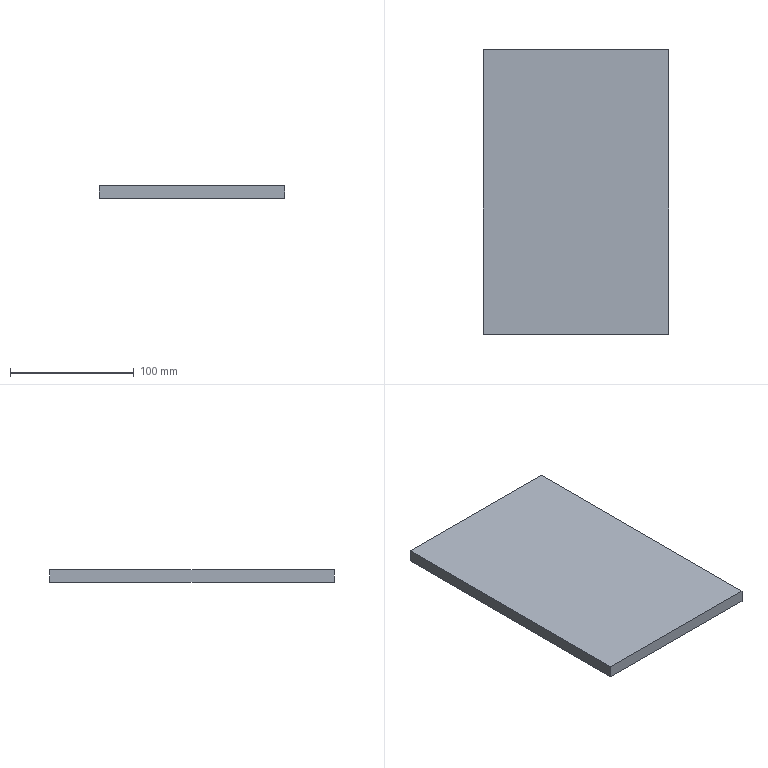Part | SolidWorks | features Extrusion 1 | 1 solid | 6 faces | box 150 x 230 x 10 mm | volume 345000 mm3 | plane 6
STEP:
#1=CARTESIAN_POINT('',(-75.,115.,-5.));
#2=VERTEX_POINT('',#1);
#3=CARTESIAN_POINT('',(-75.,-115.,-5.));
#4=VERTEX_POINT('',#3);
#5=CARTESIAN_POINT('',(-75.,-115.,-5.));
#6=DIRECTION('',(0.,-1.,0.));
#7=VECTOR('',#6,1000.);
#8=LINE('',#5,#7);
#9=EDGE_CURVE('',#2,#4,#8,.T.);
#10=ORIENTED_EDGE('',*,*,#9,.T.);
#11=CARTESIAN_POINT('',(-75.,-115.,5.));
#12=VERTEX_POINT('',#11);
#13=CARTESIAN_POINT('',(-75.,-115.,5.));
#14=DIRECTION('',(0.,0.,-1.));
#15=VECTOR('',#14,1000.);
#16=LINE('',#13,#15);
#17=EDGE_CURVE('',#12,#4,#16,.T.);
#18=ORIENTED_EDGE('',*,*,#17,.F.);
#19=CARTESIAN_POINT('',(-75.,115.,5.));
#20=VERTEX_POINT('',#19);
#21=CARTESIAN_POINT('',(-75.,-115.,5.));
#22=DIRECTION('',(0.,-1.,0.));
#23=VECTOR('',#22,1000.);
#24=LINE('',#21,#23);
#25=EDGE_CURVE('',#20,#12,#24,.T.);
#26=ORIENTED_EDGE('',*,*,#25,.F.);
#27=CARTESIAN_POINT('',(-75.,115.,5.));
#28=DIRECTION('',(0.,0.,-1.));
#29=VECTOR('',#28,1000.);
#30=LINE('',#27,#29);
#31=EDGE_CURVE('',#20,#2,#30,.T.);
#32=ORIENTED_EDGE('',*,*,#31,.T.);
#33=EDGE_LOOP('',(#10,#18,#26,#32));
#34=FACE_OUTER_BOUND('',#33,.T.);
#35=CARTESIAN_POINT('',(-75.,-115.,5.));
#36=DIRECTION('',(1.,0.,0.));
#37=DIRECTION('',(0.,0.,-1.));
#38=AXIS2_PLACEMENT_3D('',#35,#36,#37);
#39=PLANE('',#38);
#40=ADVANCED_FACE('',(#34),#39,.F.);
#41=CARTESIAN_POINT('',(75.,-115.,-5.));
#42=VERTEX_POINT('',#41);
#43=CARTESIAN_POINT('',(75.,-115.,-5.));
#44=DIRECTION('',(1.,0.,0.));
#45=VECTOR('',#44,1000.);
#46=LINE('',#43,#45);
#47=EDGE_CURVE('',#4,#42,#46,.T.);
#48=ORIENTED_EDGE('',*,*,#47,.T.);
#49=CARTESIAN_POINT('',(75.,-115.,5.));
#50=VERTEX_POINT('',#49);
#51=CARTESIAN_POINT('',(75.,-115.,5.));
#52=DIRECTION('',(0.,0.,-1.));
#53=VECTOR('',#52,1000.);
#54=LINE('',#51,#53);
#55=EDGE_CURVE('',#50,#42,#54,.T.);
#56=ORIENTED_EDGE('',*,*,#55,.F.);
#57=CARTESIAN_POINT('',(75.,-115.,5.));
#58=DIRECTION('',(1.,0.,0.));
#59=VECTOR('',#58,1000.);
#60=LINE('',#57,#59);
#61=EDGE_CURVE('',#12,#50,#60,.T.);
#62=ORIENTED_EDGE('',*,*,#61,.F.);
#63=ORIENTED_EDGE('',*,*,#17,.T.);
#64=EDGE_LOOP('',(#48,#56,#62,#63));
#65=FACE_OUTER_BOUND('',#64,.T.);
#66=CARTESIAN_POINT('',(75.,-115.,5.));
#67=DIRECTION('',(0.,1.,0.));
#68=DIRECTION('',(-1.,0.,0.));
#69=AXIS2_PLACEMENT_3D('',#66,#67,#68);
#70=PLANE('',#69);
#71=ADVANCED_FACE('',(#65),#70,.F.);
#72=CARTESIAN_POINT('',(75.,115.,-5.));
#73=VERTEX_POINT('',#72);
#74=CARTESIAN_POINT('',(75.,-115.,-5.));
#75=DIRECTION('',(0.,1.,0.));
#76=VECTOR('',#75,1000.);
#77=LINE('',#74,#76);
#78=EDGE_CURVE('',#42,#73,#77,.T.);
#79=ORIENTED_EDGE('',*,*,#78,.T.);
#80=CARTESIAN_POINT('',(75.,115.,5.));
#81=VERTEX_POINT('',#80);
#82=CARTESIAN_POINT('',(75.,115.,5.));
#83=DIRECTION('',(0.,0.,-1.));
#84=VECTOR('',#83,1000.);
#85=LINE('',#82,#84);
#86=EDGE_CURVE('',#81,#73,#85,.T.);
#87=ORIENTED_EDGE('',*,*,#86,.F.);
#88=CARTESIAN_POINT('',(75.,-115.,5.));
#89=DIRECTION('',(0.,1.,0.));
#90=VECTOR('',#89,1000.);
#91=LINE('',#88,#90);
#92=EDGE_CURVE('',#50,#81,#91,.T.);
#93=ORIENTED_EDGE('',*,*,#92,.F.);
#94=ORIENTED_EDGE('',*,*,#55,.T.);
#95=EDGE_LOOP('',(#79,#87,#93,#94));
#96=FACE_OUTER_BOUND('',#95,.T.);
#97=CARTESIAN_POINT('',(75.,-115.,5.));
#98=DIRECTION('',(-1.,0.,0.));
#99=DIRECTION('',(0.,0.,1.));
#100=AXIS2_PLACEMENT_3D('',#97,#98,#99);
#101=PLANE('',#100);
#102=ADVANCED_FACE('',(#96),#101,.F.);
#103=CARTESIAN_POINT('',(75.,115.,-5.));
#104=DIRECTION('',(-1.,0.,0.));
#105=VECTOR('',#104,1000.);
#106=LINE('',#103,#105);
#107=EDGE_CURVE('',#73,#2,#106,.T.);
#108=ORIENTED_EDGE('',*,*,#107,.T.);
#109=ORIENTED_EDGE('',*,*,#31,.F.);
#110=CARTESIAN_POINT('',(75.,115.,5.));
#111=DIRECTION('',(-1.,0.,0.));
#112=VECTOR('',#111,1000.);
#113=LINE('',#110,#112);
#114=EDGE_CURVE('',#81,#20,#113,.T.);
#115=ORIENTED_EDGE('',*,*,#114,.F.);
#116=ORIENTED_EDGE('',*,*,#86,.T.);
#117=EDGE_LOOP('',(#108,#109,#115,#116));
#118=FACE_OUTER_BOUND('',#117,.T.);
#119=CARTESIAN_POINT('',(75.,115.,5.));
#120=DIRECTION('',(0.,-1.,0.));
#121=DIRECTION('',(0.,0.,-1.));
#122=AXIS2_PLACEMENT_3D('',#119,#120,#121);
#123=PLANE('',#122);
#124=ADVANCED_FACE('',(#118),#123,.F.);
#125=ORIENTED_EDGE('',*,*,#25,.T.);
#126=ORIENTED_EDGE('',*,*,#61,.T.);
#127=ORIENTED_EDGE('',*,*,#92,.T.);
#128=ORIENTED_EDGE('',*,*,#114,.T.);
#129=EDGE_LOOP('',(#125,#126,#127,#128));
#130=FACE_OUTER_BOUND('',#129,.T.);
#131=CARTESIAN_POINT('',(0.,0.,5.));
#132=DIRECTION('',(0.,0.,1.));
#133=DIRECTION('',(1.,0.,0.));
#134=AXIS2_PLACEMENT_3D('',#131,#132,#133);
#135=PLANE('',#134);
#136=ADVANCED_FACE('',(#130),#135,.T.);
#137=ORIENTED_EDGE('',*,*,#9,.F.);
#138=ORIENTED_EDGE('',*,*,#107,.F.);
#139=ORIENTED_EDGE('',*,*,#78,.F.);
#140=ORIENTED_EDGE('',*,*,#47,.F.);
#141=EDGE_LOOP('',(#137,#138,#139,#140));
#142=FACE_OUTER_BOUND('',#141,.T.);
#143=CARTESIAN_POINT('',(0.,0.,-5.));
#144=DIRECTION('',(0.,0.,1.));
#145=DIRECTION('',(1.,0.,0.));
#146=AXIS2_PLACEMENT_3D('',#143,#144,#145);
#147=PLANE('',#146);
#148=ADVANCED_FACE('',(#142),#147,.F.);
#149=CLOSED_SHELL('',(#40,#71,#102,#124,#136,#148));
#150=MANIFOLD_SOLID_BREP('',#149);
#151=CARTESIAN_POINT('',(0.,0.,0.));
#152=DIRECTION('',(0.,0.,1.));
#153=DIRECTION('',(1.,0.,0.));
#154=AXIS2_PLACEMENT_3D('',#151,#152,#153);
#155=(LENGTH_UNIT()NAMED_UNIT(*)SI_UNIT(.MILLI.,.METRE.));
#156=UNCERTAINTY_MEASURE_WITH_UNIT(LENGTH_MEASURE(0.00001),#155,'','');
#157=(NAMED_UNIT(*)PLANE_ANGLE_UNIT()SI_UNIT($,.RADIAN.));
#158=(NAMED_UNIT(*)SI_UNIT($,.STERADIAN.)SOLID_ANGLE_UNIT());
#159=(GEOMETRIC_REPRESENTATION_CONTEXT(3)GLOBAL_UNCERTAINTY_ASSIGNED_CONTEXT((#156))GLOBAL_UNIT_ASSIGNED_CONTEXT((#155,#157,#158))REPRESENTATION_CONTEXT('',''));
#160=ADVANCED_BREP_SHAPE_REPRESENTATION('',(#150,#154),#159);